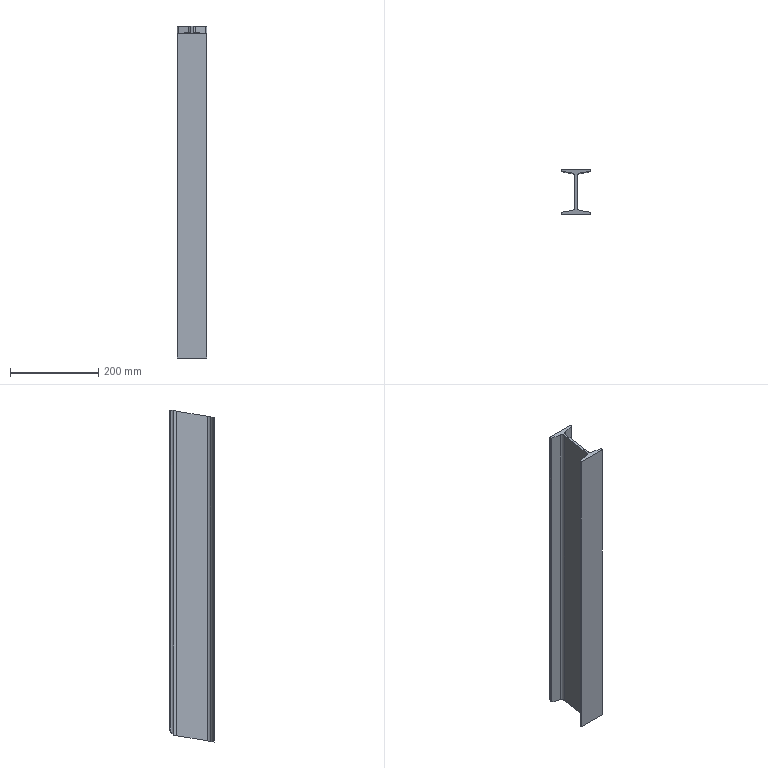Part | SolidWorks | features BaseBody 1 | 1 solid | 23 faces | box 67.6 x 101.6 x 753.5 mm | volume 1021639 mm3 | plane 15 | cylinder 8 | commonest cylinder face diameters 5.6 x4 14.8 x4
STEP:
#1=CARTESIAN_POINT('',(17.268,-1.81,2.654));
#2=VERTEX_POINT('',#1);
#3=CARTESIAN_POINT('',(17.268,68.07,14.348));
#4=VERTEX_POINT('',#3);
#5=CARTESIAN_POINT('',(17.268,-1.81,2.654));
#6=DIRECTION('',(0.,0.9863,0.165));
#7=VECTOR('',#6,1000.);
#8=LINE('',#5,#7);
#9=EDGE_CURVE('',#2,#4,#8,.T.);
#10=ORIENTED_EDGE('',*,*,#9,.T.);
#11=CARTESIAN_POINT('',(17.268,68.07,750.846));
#12=VERTEX_POINT('',#11);
#13=CARTESIAN_POINT('',(17.268,68.07,0.));
#14=DIRECTION('',(0.,0.,1.));
#15=VECTOR('',#14,1000.);
#16=LINE('',#13,#15);
#17=EDGE_CURVE('',#4,#12,#16,.T.);
#18=ORIENTED_EDGE('',*,*,#17,.T.);
#19=CARTESIAN_POINT('',(17.268,-1.81,739.152));
#20=VERTEX_POINT('',#19);
#21=CARTESIAN_POINT('',(17.268,68.07,750.846));
#22=DIRECTION('',(0.,-0.9863,-0.165));
#23=VECTOR('',#22,1000.);
#24=LINE('',#21,#23);
#25=EDGE_CURVE('',#12,#20,#24,.T.);
#26=ORIENTED_EDGE('',*,*,#25,.T.);
#27=CARTESIAN_POINT('',(17.268,-1.81,0.));
#28=DIRECTION('',(0.,0.,-1.));
#29=VECTOR('',#28,1000.);
#30=LINE('',#27,#29);
#31=EDGE_CURVE('',#20,#2,#30,.T.);
#32=ORIENTED_EDGE('',*,*,#31,.T.);
#33=EDGE_LOOP('',(#10,#18,#26,#32));
#34=FACE_OUTER_BOUND('',#33,.T.);
#35=CARTESIAN_POINT('',(17.268,68.07,0.));
#36=DIRECTION('',(1.,0.,0.));
#37=DIRECTION('',(0.,0.,-1.));
#38=AXIS2_PLACEMENT_3D('',#35,#36,#37);
#39=PLANE('',#38);
#40=ADVANCED_FACE('',(#34),#39,.T.);
#41=ORIENTED_EDGE('',*,*,#17,.F.);
#42=CARTESIAN_POINT('',(23.446,75.369,15.569));
#43=VERTEX_POINT('',#42);
#44=CARTESIAN_POINT('',(23.446,75.369,15.569));
#45=CARTESIAN_POINT('',(19.713,74.744,15.465));
#46=CARTESIAN_POINT('',(17.268,71.855,14.981));
#47=CARTESIAN_POINT('',(17.268,68.07,14.348));
#48=(BOUNDED_CURVE()B_SPLINE_CURVE(3,(#44,#45,#46,#47),.UNSPECIFIED.,.F.,.T.)B_SPLINE_CURVE_WITH_KNOTS((4,4),(0.1658,1.571),.UNSPECIFIED.)CURVE()GEOMETRIC_REPRESENTATION_ITEM()RATIONAL_B_SPLINE_CURVE((1.,0.8422,0.8422,1.))REPRESENTATION_ITEM(''));
#49=EDGE_CURVE('',#43,#4,#48,.T.);
#50=ORIENTED_EDGE('',*,*,#49,.F.);
#51=CARTESIAN_POINT('',(23.446,75.369,752.067));
#52=VERTEX_POINT('',#51);
#53=CARTESIAN_POINT('',(23.446,75.369,0.));
#54=DIRECTION('',(0.,0.,-1.));
#55=VECTOR('',#54,1000.);
#56=LINE('',#53,#55);
#57=EDGE_CURVE('',#52,#43,#56,.T.);
#58=ORIENTED_EDGE('',*,*,#57,.F.);
#59=CARTESIAN_POINT('',(17.268,68.07,750.846));
#60=CARTESIAN_POINT('',(17.268,71.855,751.479));
#61=CARTESIAN_POINT('',(19.713,74.744,751.963));
#62=CARTESIAN_POINT('',(23.446,75.369,752.067));
#63=(BOUNDED_CURVE()B_SPLINE_CURVE(3,(#59,#60,#61,#62),.UNSPECIFIED.,.F.,.F.)B_SPLINE_CURVE_WITH_KNOTS((4,4),(4.712,6.117),.UNSPECIFIED.)CURVE()GEOMETRIC_REPRESENTATION_ITEM()RATIONAL_B_SPLINE_CURVE((1.,0.8422,0.8422,1.))REPRESENTATION_ITEM(''));
#64=EDGE_CURVE('',#12,#52,#63,.T.);
#65=ORIENTED_EDGE('',*,*,#64,.F.);
#66=EDGE_LOOP('',(#41,#50,#58,#65));
#67=FACE_OUTER_BOUND('',#66,.T.);
#68=CARTESIAN_POINT('',(24.668,68.07,0.));
#69=DIRECTION('',(0.,0.,1.));
#70=DIRECTION('',(1.,0.,0.));
#71=AXIS2_PLACEMENT_3D('',#68,#69,#70);
#72=CYLINDRICAL_SURFACE('',#71,7.4);
#73=ADVANCED_FACE('',(#67),#72,.F.);
#74=CARTESIAN_POINT('',(12.468,68.07,14.348));
#75=VERTEX_POINT('',#74);
#76=CARTESIAN_POINT('',(6.289,75.369,15.569));
#77=VERTEX_POINT('',#76);
#78=CARTESIAN_POINT('',(12.468,68.07,14.348));
#79=CARTESIAN_POINT('',(12.468,71.855,14.981));
#80=CARTESIAN_POINT('',(10.022,74.744,15.465));
#81=CARTESIAN_POINT('',(6.289,75.369,15.569));
#82=(BOUNDED_CURVE()B_SPLINE_CURVE(3,(#78,#79,#80,#81),.UNSPECIFIED.,.F.,.T.)B_SPLINE_CURVE_WITH_KNOTS((4,4),(4.712,6.117),.UNSPECIFIED.)CURVE()GEOMETRIC_REPRESENTATION_ITEM()RATIONAL_B_SPLINE_CURVE((1.,0.8422,0.8422,1.))REPRESENTATION_ITEM(''));
#83=EDGE_CURVE('',#75,#77,#82,.T.);
#84=ORIENTED_EDGE('',*,*,#83,.T.);
#85=CARTESIAN_POINT('',(2.278,76.04,15.682));
#86=VERTEX_POINT('',#85);
#87=CARTESIAN_POINT('',(6.289,75.369,15.569));
#88=DIRECTION('',(-0.9859,0.165,0.02761));
#89=VECTOR('',#88,1000.);
#90=LINE('',#87,#89);
#91=EDGE_CURVE('',#77,#86,#90,.T.);
#92=ORIENTED_EDGE('',*,*,#91,.T.);
#93=CARTESIAN_POINT('',(27.457,76.04,15.682));
#94=VERTEX_POINT('',#93);
#95=CARTESIAN_POINT('',(-2.032,76.04,15.682));
#96=DIRECTION('',(1.,0.,0.));
#97=VECTOR('',#96,1000.);
#98=LINE('',#95,#97);
#99=EDGE_CURVE('',#86,#94,#98,.T.);
#100=ORIENTED_EDGE('',*,*,#99,.T.);
#101=CARTESIAN_POINT('',(27.457,76.04,15.682));
#102=DIRECTION('',(-0.9859,-0.165,-0.02761));
#103=VECTOR('',#102,1000.);
#104=LINE('',#101,#103);
#105=EDGE_CURVE('',#94,#43,#104,.T.);
#106=ORIENTED_EDGE('',*,*,#105,.T.);
#107=ORIENTED_EDGE('',*,*,#49,.T.);
#108=ORIENTED_EDGE('',*,*,#9,.F.);
#109=CARTESIAN_POINT('',(23.446,-9.108,1.433));
#110=VERTEX_POINT('',#109);
#111=CARTESIAN_POINT('',(17.268,-1.81,2.654));
#112=CARTESIAN_POINT('',(17.268,-5.595,2.021));
#113=CARTESIAN_POINT('',(19.713,-8.484,1.537));
#114=CARTESIAN_POINT('',(23.446,-9.108,1.433));
#115=(BOUNDED_CURVE()B_SPLINE_CURVE(3,(#111,#112,#113,#114),.UNSPECIFIED.,.F.,.F.)B_SPLINE_CURVE_WITH_KNOTS((4,4),(1.571,2.976),.UNSPECIFIED.)CURVE()GEOMETRIC_REPRESENTATION_ITEM()RATIONAL_B_SPLINE_CURVE((1.,0.8422,0.8422,1.))REPRESENTATION_ITEM(''));
#116=EDGE_CURVE('',#2,#110,#115,.T.);
#117=ORIENTED_EDGE('',*,*,#116,.T.);
#118=CARTESIAN_POINT('',(46.33,-12.938,0.7919));
#119=VERTEX_POINT('',#118);
#120=CARTESIAN_POINT('',(23.446,-9.108,1.433));
#121=DIRECTION('',(0.9859,-0.165,-0.02761));
#122=VECTOR('',#121,1000.);
#123=LINE('',#120,#122);
#124=EDGE_CURVE('',#110,#119,#123,.T.);
#125=ORIENTED_EDGE('',*,*,#124,.T.);
#126=CARTESIAN_POINT('',(48.668,-15.699,0.3297));
#127=VERTEX_POINT('',#126);
#128=CARTESIAN_POINT('',(46.33,-12.938,0.7919));
#129=CARTESIAN_POINT('',(47.742,-13.174,0.7523));
#130=CARTESIAN_POINT('',(48.668,-14.267,0.5694));
#131=CARTESIAN_POINT('',(48.668,-15.699,0.3297));
#132=(BOUNDED_CURVE()B_SPLINE_CURVE(3,(#128,#129,#130,#131),.UNSPECIFIED.,.F.,.F.)B_SPLINE_CURVE_WITH_KNOTS((4,4),(0.1658,1.571),.UNSPECIFIED.)CURVE()GEOMETRIC_REPRESENTATION_ITEM()RATIONAL_B_SPLINE_CURVE((1.,0.8422,0.8422,1.))REPRESENTATION_ITEM(''));
#133=EDGE_CURVE('',#119,#127,#132,.T.);
#134=ORIENTED_EDGE('',*,*,#133,.T.);
#135=CARTESIAN_POINT('',(48.668,-17.67,0.));
#136=VERTEX_POINT('',#135);
#137=CARTESIAN_POINT('',(48.668,33.13,8.501));
#138=DIRECTION('',(0.,-0.9863,-0.165));
#139=VECTOR('',#138,1000.);
#140=LINE('',#137,#139);
#141=EDGE_CURVE('',#127,#136,#140,.T.);
#142=ORIENTED_EDGE('',*,*,#141,.T.);
#143=CARTESIAN_POINT('',(-18.932,-17.67,0.));
#144=VERTEX_POINT('',#143);
#145=CARTESIAN_POINT('',(-2.032,-17.67,0.));
#146=DIRECTION('',(-1.,0.,0.));
#147=VECTOR('',#146,1000.);
#148=LINE('',#145,#147);
#149=EDGE_CURVE('',#136,#144,#148,.T.);
#150=ORIENTED_EDGE('',*,*,#149,.T.);
#151=CARTESIAN_POINT('',(-18.932,-15.699,0.3297));
#152=VERTEX_POINT('',#151);
#153=CARTESIAN_POINT('',(-18.932,33.13,8.501));
#154=DIRECTION('',(0.,0.9863,0.165));
#155=VECTOR('',#154,1000.);
#156=LINE('',#153,#155);
#157=EDGE_CURVE('',#144,#152,#156,.T.);
#158=ORIENTED_EDGE('',*,*,#157,.T.);
#159=CARTESIAN_POINT('',(-16.594,-12.938,0.7919));
#160=VERTEX_POINT('',#159);
#161=CARTESIAN_POINT('',(-18.932,-15.699,0.3297));
#162=CARTESIAN_POINT('',(-18.932,-14.267,0.5694));
#163=CARTESIAN_POINT('',(-18.007,-13.174,0.7523));
#164=CARTESIAN_POINT('',(-16.594,-12.938,0.7919));
#165=(BOUNDED_CURVE()B_SPLINE_CURVE(3,(#161,#162,#163,#164),.UNSPECIFIED.,.F.,.F.)B_SPLINE_CURVE_WITH_KNOTS((4,4),(4.712,6.117),.UNSPECIFIED.)CURVE()GEOMETRIC_REPRESENTATION_ITEM()RATIONAL_B_SPLINE_CURVE((1.,0.8422,0.8422,1.))REPRESENTATION_ITEM(''));
#166=EDGE_CURVE('',#152,#160,#165,.T.);
#167=ORIENTED_EDGE('',*,*,#166,.T.);
#168=CARTESIAN_POINT('',(6.289,-9.108,1.433));
#169=VERTEX_POINT('',#168);
#170=CARTESIAN_POINT('',(-16.594,-12.938,0.7919));
#171=DIRECTION('',(0.9859,0.165,0.02761));
#172=VECTOR('',#171,1000.);
#173=LINE('',#170,#172);
#174=EDGE_CURVE('',#160,#169,#173,.T.);
#175=ORIENTED_EDGE('',*,*,#174,.T.);
#176=CARTESIAN_POINT('',(12.468,-1.81,2.654));
#177=VERTEX_POINT('',#176);
#178=CARTESIAN_POINT('',(6.289,-9.108,1.433));
#179=CARTESIAN_POINT('',(10.022,-8.484,1.537));
#180=CARTESIAN_POINT('',(12.468,-5.595,2.021));
#181=CARTESIAN_POINT('',(12.468,-1.81,2.654));
#182=(BOUNDED_CURVE()B_SPLINE_CURVE(3,(#178,#179,#180,#181),.UNSPECIFIED.,.F.,.T.)B_SPLINE_CURVE_WITH_KNOTS((4,4),(3.307,4.712),.UNSPECIFIED.)CURVE()GEOMETRIC_REPRESENTATION_ITEM()RATIONAL_B_SPLINE_CURVE((1.,0.8422,0.8422,1.))REPRESENTATION_ITEM(''));
#183=EDGE_CURVE('',#169,#177,#182,.T.);
#184=ORIENTED_EDGE('',*,*,#183,.T.);
#185=CARTESIAN_POINT('',(12.468,33.13,8.501));
#186=DIRECTION('',(0.,0.9863,0.165));
#187=VECTOR('',#186,1000.);
#188=LINE('',#185,#187);
#189=EDGE_CURVE('',#177,#75,#188,.T.);
#190=ORIENTED_EDGE('',*,*,#189,.T.);
#191=EDGE_LOOP('',(#84,#92,#100,#106,#107,#108,#117,#125,#134,#142,#150,#158,#167,#175,#184,#190));
#192=FACE_OUTER_BOUND('',#191,.T.);
#193=CARTESIAN_POINT('',(-2.032,33.13,8.501));
#194=DIRECTION('',(0.,0.165,-0.9863));
#195=DIRECTION('',(0.,0.9863,0.165));
#196=AXIS2_PLACEMENT_3D('',#193,#194,#195);
#197=PLANE('',#196);
#198=ADVANCED_FACE('',(#192),#197,.T.);
#199=CARTESIAN_POINT('',(23.446,-9.108,737.931));
#200=VERTEX_POINT('',#199);
#201=CARTESIAN_POINT('',(23.446,-9.108,0.));
#202=DIRECTION('',(0.,0.,1.));
#203=VECTOR('',#202,1000.);
#204=LINE('',#201,#203);
#205=EDGE_CURVE('',#110,#200,#204,.T.);
#206=ORIENTED_EDGE('',*,*,#205,.F.);
#207=ORIENTED_EDGE('',*,*,#116,.F.);
#208=ORIENTED_EDGE('',*,*,#31,.F.);
#209=CARTESIAN_POINT('',(23.446,-9.108,737.931));
#210=CARTESIAN_POINT('',(19.713,-8.484,738.035));
#211=CARTESIAN_POINT('',(17.268,-5.595,738.519));
#212=CARTESIAN_POINT('',(17.268,-1.81,739.152));
#213=(BOUNDED_CURVE()B_SPLINE_CURVE(3,(#209,#210,#211,#212),.UNSPECIFIED.,.F.,.T.)B_SPLINE_CURVE_WITH_KNOTS((4,4),(3.307,4.712),.UNSPECIFIED.)CURVE()GEOMETRIC_REPRESENTATION_ITEM()RATIONAL_B_SPLINE_CURVE((1.,0.8422,0.8422,1.))REPRESENTATION_ITEM(''));
#214=EDGE_CURVE('',#200,#20,#213,.T.);
#215=ORIENTED_EDGE('',*,*,#214,.F.);
#216=EDGE_LOOP('',(#206,#207,#208,#215));
#217=FACE_OUTER_BOUND('',#216,.T.);
#218=CARTESIAN_POINT('',(24.668,-1.81,0.));
#219=DIRECTION('',(0.,0.,1.));
#220=DIRECTION('',(1.,0.,0.));
#221=AXIS2_PLACEMENT_3D('',#218,#219,#220);
#222=CYLINDRICAL_SURFACE('',#221,7.4);
#223=ADVANCED_FACE('',(#217),#222,.F.);
#224=CARTESIAN_POINT('',(6.289,-9.108,737.931));
#225=VERTEX_POINT('',#224);
#226=CARTESIAN_POINT('',(-16.594,-12.938,737.29));
#227=VERTEX_POINT('',#226);
#228=CARTESIAN_POINT('',(6.289,-9.108,737.931));
#229=DIRECTION('',(-0.9859,-0.165,-0.02761));
#230=VECTOR('',#229,1000.);
#231=LINE('',#228,#230);
#232=EDGE_CURVE('',#225,#227,#231,.T.);
#233=ORIENTED_EDGE('',*,*,#232,.T.);
#234=CARTESIAN_POINT('',(-18.932,-15.699,736.828));
#235=VERTEX_POINT('',#234);
#236=CARTESIAN_POINT('',(-16.594,-12.938,737.29));
#237=CARTESIAN_POINT('',(-18.007,-13.174,737.25));
#238=CARTESIAN_POINT('',(-18.932,-14.267,737.067));
#239=CARTESIAN_POINT('',(-18.932,-15.699,736.828));
#240=(BOUNDED_CURVE()B_SPLINE_CURVE(3,(#236,#237,#238,#239),.UNSPECIFIED.,.F.,.T.)B_SPLINE_CURVE_WITH_KNOTS((4,4),(0.1658,1.571),.UNSPECIFIED.)CURVE()GEOMETRIC_REPRESENTATION_ITEM()RATIONAL_B_SPLINE_CURVE((1.,0.8422,0.8422,1.))REPRESENTATION_ITEM(''));
#241=EDGE_CURVE('',#227,#235,#240,.T.);
#242=ORIENTED_EDGE('',*,*,#241,.T.);
#243=CARTESIAN_POINT('',(-18.932,-17.67,736.498));
#244=VERTEX_POINT('',#243);
#245=CARTESIAN_POINT('',(-18.932,33.13,744.999));
#246=DIRECTION('',(0.,-0.9863,-0.165));
#247=VECTOR('',#246,1000.);
#248=LINE('',#245,#247);
#249=EDGE_CURVE('',#235,#244,#248,.T.);
#250=ORIENTED_EDGE('',*,*,#249,.T.);
#251=CARTESIAN_POINT('',(48.668,-17.67,736.498));
#252=VERTEX_POINT('',#251);
#253=CARTESIAN_POINT('',(31.768,-17.67,736.498));
#254=DIRECTION('',(1.,0.,0.));
#255=VECTOR('',#254,1000.);
#256=LINE('',#253,#255);
#257=EDGE_CURVE('',#244,#252,#256,.T.);
#258=ORIENTED_EDGE('',*,*,#257,.T.);
#259=CARTESIAN_POINT('',(48.668,-15.699,736.828));
#260=VERTEX_POINT('',#259);
#261=CARTESIAN_POINT('',(48.668,33.13,744.999));
#262=DIRECTION('',(0.,0.9863,0.165));
#263=VECTOR('',#262,1000.);
#264=LINE('',#261,#263);
#265=EDGE_CURVE('',#252,#260,#264,.T.);
#266=ORIENTED_EDGE('',*,*,#265,.T.);
#267=CARTESIAN_POINT('',(46.33,-12.938,737.29));
#268=VERTEX_POINT('',#267);
#269=CARTESIAN_POINT('',(48.668,-15.699,736.828));
#270=CARTESIAN_POINT('',(48.668,-14.267,737.067));
#271=CARTESIAN_POINT('',(47.742,-13.174,737.25));
#272=CARTESIAN_POINT('',(46.33,-12.938,737.29));
#273=(BOUNDED_CURVE()B_SPLINE_CURVE(3,(#269,#270,#271,#272),.UNSPECIFIED.,.F.,.T.)B_SPLINE_CURVE_WITH_KNOTS((4,4),(4.712,6.117),.UNSPECIFIED.)CURVE()GEOMETRIC_REPRESENTATION_ITEM()RATIONAL_B_SPLINE_CURVE((1.,0.8422,0.8422,1.))REPRESENTATION_ITEM(''));
#274=EDGE_CURVE('',#260,#268,#273,.T.);
#275=ORIENTED_EDGE('',*,*,#274,.T.);
#276=CARTESIAN_POINT('',(46.33,-12.938,737.29));
#277=DIRECTION('',(-0.9859,0.165,0.02761));
#278=VECTOR('',#277,1000.);
#279=LINE('',#276,#278);
#280=EDGE_CURVE('',#268,#200,#279,.T.);
#281=ORIENTED_EDGE('',*,*,#280,.T.);
#282=ORIENTED_EDGE('',*,*,#214,.T.);
#283=ORIENTED_EDGE('',*,*,#25,.F.);
#284=ORIENTED_EDGE('',*,*,#64,.T.);
#285=CARTESIAN_POINT('',(46.33,79.198,752.708));
#286=VERTEX_POINT('',#285);
#287=CARTESIAN_POINT('',(23.446,75.369,752.067));
#288=DIRECTION('',(0.9859,0.165,0.02761));
#289=VECTOR('',#288,1000.);
#290=LINE('',#287,#289);
#291=EDGE_CURVE('',#52,#286,#290,.T.);
#292=ORIENTED_EDGE('',*,*,#291,.T.);
#293=CARTESIAN_POINT('',(48.668,81.96,753.17));
#294=VERTEX_POINT('',#293);
#295=CARTESIAN_POINT('',(46.33,79.198,752.708));
#296=CARTESIAN_POINT('',(47.742,79.434,752.748));
#297=CARTESIAN_POINT('',(48.668,80.527,752.931));
#298=CARTESIAN_POINT('',(48.668,81.96,753.17));
#299=(BOUNDED_CURVE()B_SPLINE_CURVE(3,(#295,#296,#297,#298),.UNSPECIFIED.,.F.,.T.)B_SPLINE_CURVE_WITH_KNOTS((4,4),(3.307,4.712),.UNSPECIFIED.)CURVE()GEOMETRIC_REPRESENTATION_ITEM()RATIONAL_B_SPLINE_CURVE((1.,0.8422,0.8422,1.))REPRESENTATION_ITEM(''));
#300=EDGE_CURVE('',#286,#294,#299,.T.);
#301=ORIENTED_EDGE('',*,*,#300,.T.);
#302=CARTESIAN_POINT('',(48.668,83.93,753.5));
#303=VERTEX_POINT('',#302);
#304=CARTESIAN_POINT('',(48.668,33.13,744.999));
#305=DIRECTION('',(0.,0.9863,0.165));
#306=VECTOR('',#305,1000.);
#307=LINE('',#304,#306);
#308=EDGE_CURVE('',#294,#303,#307,.T.);
#309=ORIENTED_EDGE('',*,*,#308,.T.);
#310=CARTESIAN_POINT('',(-18.932,83.93,753.5));
#311=VERTEX_POINT('',#310);
#312=CARTESIAN_POINT('',(31.768,83.93,753.5));
#313=DIRECTION('',(-1.,0.,0.));
#314=VECTOR('',#313,1000.);
#315=LINE('',#312,#314);
#316=EDGE_CURVE('',#303,#311,#315,.T.);
#317=ORIENTED_EDGE('',*,*,#316,.T.);
#318=CARTESIAN_POINT('',(-18.932,81.96,753.17));
#319=VERTEX_POINT('',#318);
#320=CARTESIAN_POINT('',(-18.932,33.13,744.999));
#321=DIRECTION('',(0.,-0.9863,-0.165));
#322=VECTOR('',#321,1000.);
#323=LINE('',#320,#322);
#324=EDGE_CURVE('',#311,#319,#323,.T.);
#325=ORIENTED_EDGE('',*,*,#324,.T.);
#326=CARTESIAN_POINT('',(-16.594,79.198,752.708));
#327=VERTEX_POINT('',#326);
#328=CARTESIAN_POINT('',(-18.932,81.96,753.17));
#329=CARTESIAN_POINT('',(-18.932,80.527,752.931));
#330=CARTESIAN_POINT('',(-18.007,79.434,752.748));
#331=CARTESIAN_POINT('',(-16.594,79.198,752.708));
#332=(BOUNDED_CURVE()B_SPLINE_CURVE(3,(#328,#329,#330,#331),.UNSPECIFIED.,.F.,.T.)B_SPLINE_CURVE_WITH_KNOTS((4,4),(1.571,2.976),.UNSPECIFIED.)CURVE()GEOMETRIC_REPRESENTATION_ITEM()RATIONAL_B_SPLINE_CURVE((1.,0.8422,0.8422,1.))REPRESENTATION_ITEM(''));
#333=EDGE_CURVE('',#319,#327,#332,.T.);
#334=ORIENTED_EDGE('',*,*,#333,.T.);
#335=CARTESIAN_POINT('',(6.289,75.369,752.067));
#336=VERTEX_POINT('',#335);
#337=CARTESIAN_POINT('',(-16.594,79.198,752.708));
#338=DIRECTION('',(0.9859,-0.165,-0.02761));
#339=VECTOR('',#338,1000.);
#340=LINE('',#337,#339);
#341=EDGE_CURVE('',#327,#336,#340,.T.);
#342=ORIENTED_EDGE('',*,*,#341,.T.);
#343=CARTESIAN_POINT('',(12.468,68.07,750.846));
#344=VERTEX_POINT('',#343);
#345=CARTESIAN_POINT('',(6.289,75.369,752.067));
#346=CARTESIAN_POINT('',(10.022,74.744,751.963));
#347=CARTESIAN_POINT('',(12.468,71.855,751.479));
#348=CARTESIAN_POINT('',(12.468,68.07,750.846));
#349=(BOUNDED_CURVE()B_SPLINE_CURVE(3,(#345,#346,#347,#348),.UNSPECIFIED.,.F.,.T.)B_SPLINE_CURVE_WITH_KNOTS((4,4),(0.1658,1.571),.UNSPECIFIED.)CURVE()GEOMETRIC_REPRESENTATION_ITEM()RATIONAL_B_SPLINE_CURVE((1.,0.8422,0.8422,1.))REPRESENTATION_ITEM(''));
#350=EDGE_CURVE('',#336,#344,#349,.T.);
#351=ORIENTED_EDGE('',*,*,#350,.T.);
#352=CARTESIAN_POINT('',(12.468,-1.81,739.152));
#353=VERTEX_POINT('',#352);
#354=CARTESIAN_POINT('',(12.468,33.13,744.999));
#355=DIRECTION('',(0.,-0.9863,-0.165));
#356=VECTOR('',#355,1000.);
#357=LINE('',#354,#356);
#358=EDGE_CURVE('',#344,#353,#357,.T.);
#359=ORIENTED_EDGE('',*,*,#358,.T.);
#360=CARTESIAN_POINT('',(12.468,-1.81,739.152));
#361=CARTESIAN_POINT('',(12.468,-5.595,738.519));
#362=CARTESIAN_POINT('',(10.022,-8.484,738.035));
#363=CARTESIAN_POINT('',(6.289,-9.108,737.931));
#364=(BOUNDED_CURVE()B_SPLINE_CURVE(3,(#360,#361,#362,#363),.UNSPECIFIED.,.F.,.T.)B_SPLINE_CURVE_WITH_KNOTS((4,4),(1.571,2.976),.UNSPECIFIED.)CURVE()GEOMETRIC_REPRESENTATION_ITEM()RATIONAL_B_SPLINE_CURVE((1.,0.8422,0.8422,1.))REPRESENTATION_ITEM(''));
#365=EDGE_CURVE('',#353,#225,#364,.T.);
#366=ORIENTED_EDGE('',*,*,#365,.T.);
#367=EDGE_LOOP('',(#233,#242,#250,#258,#266,#275,#281,#282,#283,#284,#292,#301,#309,#317,#325,#334,#342,#351,#359,#366));
#368=FACE_OUTER_BOUND('',#367,.T.);
#369=CARTESIAN_POINT('',(31.768,33.13,744.999));
#370=DIRECTION('',(0.,-0.165,0.9863));
#371=DIRECTION('',(0.,-0.9863,-0.165));
#372=AXIS2_PLACEMENT_3D('',#369,#370,#371);
#373=PLANE('',#372);
#374=ADVANCED_FACE('',(#368),#373,.T.);
#375=ORIENTED_EDGE('',*,*,#57,.T.);
#376=ORIENTED_EDGE('',*,*,#105,.F.);
#377=CARTESIAN_POINT('',(46.33,79.198,19.412));
#378=VERTEX_POINT('',#377);
#379=CARTESIAN_POINT('',(27.457,76.04,15.682));
#380=DIRECTION('',(0.9681,0.162,0.1914));
#381=VECTOR('',#380,1000.);
#382=LINE('',#379,#381);
#383=EDGE_CURVE('',#94,#378,#382,.T.);
#384=ORIENTED_EDGE('',*,*,#383,.T.);
#385=CARTESIAN_POINT('',(46.33,79.198,0.));
#386=DIRECTION('',(0.,0.,1.));
#387=VECTOR('',#386,1000.);
#388=LINE('',#385,#387);
#389=EDGE_CURVE('',#378,#286,#388,.T.);
#390=ORIENTED_EDGE('',*,*,#389,.T.);
#391=ORIENTED_EDGE('',*,*,#291,.F.);
#392=EDGE_LOOP('',(#375,#376,#384,#390,#391));
#393=FACE_OUTER_BOUND('',#392,.T.);
#394=CARTESIAN_POINT('',(46.33,79.198,0.));
#395=DIRECTION('',(0.165,-0.9863,0.));
#396=DIRECTION('',(0.9863,0.165,0.));
#397=AXIS2_PLACEMENT_3D('',#394,#395,#396);
#398=PLANE('',#397);
#399=ADVANCED_FACE('',(#393),#398,.T.);
#400=ORIENTED_EDGE('',*,*,#341,.F.);
#401=CARTESIAN_POINT('',(-16.594,79.198,19.412));
#402=VERTEX_POINT('',#401);
#403=CARTESIAN_POINT('',(-16.594,79.198,0.));
#404=DIRECTION('',(0.,0.,-1.));
#405=VECTOR('',#404,1000.);
#406=LINE('',#403,#405);
#407=EDGE_CURVE('',#327,#402,#406,.T.);
#408=ORIENTED_EDGE('',*,*,#407,.T.);
#409=CARTESIAN_POINT('',(-16.594,79.198,19.412));
#410=DIRECTION('',(0.9681,-0.162,-0.1914));
#411=VECTOR('',#410,1000.);
#412=LINE('',#409,#411);
#413=EDGE_CURVE('',#402,#86,#412,.T.);
#414=ORIENTED_EDGE('',*,*,#413,.T.);
#415=ORIENTED_EDGE('',*,*,#91,.F.);
#416=CARTESIAN_POINT('',(6.289,75.369,0.));
#417=DIRECTION('',(0.,0.,1.));
#418=VECTOR('',#417,1000.);
#419=LINE('',#416,#418);
#420=EDGE_CURVE('',#77,#336,#419,.T.);
#421=ORIENTED_EDGE('',*,*,#420,.T.);
#422=EDGE_LOOP('',(#400,#408,#414,#415,#421));
#423=FACE_OUTER_BOUND('',#422,.T.);
#424=CARTESIAN_POINT('',(6.289,75.369,0.));
#425=DIRECTION('',(-0.165,-0.9863,0.));
#426=DIRECTION('',(0.9863,-0.165,0.));
#427=AXIS2_PLACEMENT_3D('',#424,#425,#426);
#428=PLANE('',#427);
#429=ADVANCED_FACE('',(#423),#428,.T.);
#430=ORIENTED_EDGE('',*,*,#420,.F.);
#431=ORIENTED_EDGE('',*,*,#83,.F.);
#432=CARTESIAN_POINT('',(12.468,68.07,0.));
#433=DIRECTION('',(0.,0.,-1.));
#434=VECTOR('',#433,1000.);
#435=LINE('',#432,#434);
#436=EDGE_CURVE('',#344,#75,#435,.T.);
#437=ORIENTED_EDGE('',*,*,#436,.F.);
#438=ORIENTED_EDGE('',*,*,#350,.F.);
#439=EDGE_LOOP('',(#430,#431,#437,#438));
#440=FACE_OUTER_BOUND('',#439,.T.);
#441=CARTESIAN_POINT('',(5.068,68.07,0.));
#442=DIRECTION('',(0.,0.,1.));
#443=DIRECTION('',(1.,0.,0.));
#444=AXIS2_PLACEMENT_3D('',#441,#442,#443);
#445=CYLINDRICAL_SURFACE('',#444,7.4);
#446=ADVANCED_FACE('',(#440),#445,.F.);
#447=ORIENTED_EDGE('',*,*,#189,.F.);
#448=CARTESIAN_POINT('',(12.468,-1.81,0.));
#449=DIRECTION('',(0.,0.,1.));
#450=VECTOR('',#449,1000.);
#451=LINE('',#448,#450);
#452=EDGE_CURVE('',#177,#353,#451,.T.);
#453=ORIENTED_EDGE('',*,*,#452,.T.);
#454=ORIENTED_EDGE('',*,*,#358,.F.);
#455=ORIENTED_EDGE('',*,*,#436,.T.);
#456=EDGE_LOOP('',(#447,#453,#454,#455));
#457=FACE_OUTER_BOUND('',#456,.T.);
#458=CARTESIAN_POINT('',(12.468,-1.81,0.));
#459=DIRECTION('',(-1.,0.,0.));
#460=DIRECTION('',(0.,0.,1.));
#461=AXIS2_PLACEMENT_3D('',#458,#459,#460);
#462=PLANE('',#461);
#463=ADVANCED_FACE('',(#457),#462,.T.);
#464=ORIENTED_EDGE('',*,*,#452,.F.);
#465=ORIENTED_EDGE('',*,*,#183,.F.);
#466=CARTESIAN_POINT('',(6.289,-9.108,0.));
#467=DIRECTION('',(0.,0.,-1.));
#468=VECTOR('',#467,1000.);
#469=LINE('',#466,#468);
#470=EDGE_CURVE('',#225,#169,#469,.T.);
#471=ORIENTED_EDGE('',*,*,#470,.F.);
#472=ORIENTED_EDGE('',*,*,#365,.F.);
#473=EDGE_LOOP('',(#464,#465,#471,#472));
#474=FACE_OUTER_BOUND('',#473,.T.);
#475=CARTESIAN_POINT('',(5.068,-1.81,0.));
#476=DIRECTION('',(0.,0.,1.));
#477=DIRECTION('',(1.,0.,0.));
#478=AXIS2_PLACEMENT_3D('',#475,#476,#477);
#479=CYLINDRICAL_SURFACE('',#478,7.4);
#480=ADVANCED_FACE('',(#474),#479,.F.);
#481=ORIENTED_EDGE('',*,*,#174,.F.);
#482=CARTESIAN_POINT('',(-16.594,-12.938,0.));
#483=DIRECTION('',(0.,0.,1.));
#484=VECTOR('',#483,1000.);
#485=LINE('',#482,#484);
#486=EDGE_CURVE('',#160,#227,#485,.T.);
#487=ORIENTED_EDGE('',*,*,#486,.T.);
#488=ORIENTED_EDGE('',*,*,#232,.F.);
#489=ORIENTED_EDGE('',*,*,#470,.T.);
#490=EDGE_LOOP('',(#481,#487,#488,#489));
#491=FACE_OUTER_BOUND('',#490,.T.);
#492=CARTESIAN_POINT('',(-16.594,-12.938,0.));
#493=DIRECTION('',(-0.165,0.9863,0.));
#494=DIRECTION('',(-0.9863,-0.165,0.));
#495=AXIS2_PLACEMENT_3D('',#492,#493,#494);
#496=PLANE('',#495);
#497=ADVANCED_FACE('',(#491),#496,.T.);
#498=ORIENTED_EDGE('',*,*,#166,.F.);
#499=CARTESIAN_POINT('',(-18.932,-15.699,0.));
#500=DIRECTION('',(0.,0.,1.));
#501=VECTOR('',#500,1000.);
#502=LINE('',#499,#501);
#503=EDGE_CURVE('',#152,#235,#502,.T.);
#504=ORIENTED_EDGE('',*,*,#503,.T.);
#505=ORIENTED_EDGE('',*,*,#241,.F.);
#506=ORIENTED_EDGE('',*,*,#486,.F.);
#507=EDGE_LOOP('',(#498,#504,#505,#506));
#508=FACE_OUTER_BOUND('',#507,.T.);
#509=CARTESIAN_POINT('',(-16.132,-15.699,0.));
#510=DIRECTION('',(0.,0.,1.));
#511=DIRECTION('',(1.,0.,0.));
#512=AXIS2_PLACEMENT_3D('',#509,#510,#511);
#513=CYLINDRICAL_SURFACE('',#512,2.8);
#514=ADVANCED_FACE('',(#508),#513,.T.);
#515=ORIENTED_EDGE('',*,*,#157,.F.);
#516=CARTESIAN_POINT('',(-18.932,-17.67,0.));
#517=DIRECTION('',(0.,0.,1.));
#518=VECTOR('',#517,1000.);
#519=LINE('',#516,#518);
#520=EDGE_CURVE('',#144,#244,#519,.T.);
#521=ORIENTED_EDGE('',*,*,#520,.T.);
#522=ORIENTED_EDGE('',*,*,#249,.F.);
#523=ORIENTED_EDGE('',*,*,#503,.F.);
#524=EDGE_LOOP('',(#515,#521,#522,#523));
#525=FACE_OUTER_BOUND('',#524,.T.);
#526=CARTESIAN_POINT('',(-18.932,-17.67,0.));
#527=DIRECTION('',(-1.,0.,0.));
#528=DIRECTION('',(0.,0.,1.));
#529=AXIS2_PLACEMENT_3D('',#526,#527,#528);
#530=PLANE('',#529);
#531=ADVANCED_FACE('',(#525),#530,.T.);
#532=ORIENTED_EDGE('',*,*,#149,.F.);
#533=CARTESIAN_POINT('',(48.668,-17.67,0.));
#534=DIRECTION('',(0.,0.,1.));
#535=VECTOR('',#534,1000.);
#536=LINE('',#533,#535);
#537=EDGE_CURVE('',#136,#252,#536,.T.);
#538=ORIENTED_EDGE('',*,*,#537,.T.);
#539=ORIENTED_EDGE('',*,*,#257,.F.);
#540=ORIENTED_EDGE('',*,*,#520,.F.);
#541=EDGE_LOOP('',(#532,#538,#539,#540));
#542=FACE_OUTER_BOUND('',#541,.T.);
#543=CARTESIAN_POINT('',(48.668,-17.67,0.));
#544=DIRECTION('',(0.,-1.,0.));
#545=DIRECTION('',(0.,0.,-1.));
#546=AXIS2_PLACEMENT_3D('',#543,#544,#545);
#547=PLANE('',#546);
#548=ADVANCED_FACE('',(#542),#547,.T.);
#549=ORIENTED_EDGE('',*,*,#141,.F.);
#550=CARTESIAN_POINT('',(48.668,-15.699,0.));
#551=DIRECTION('',(0.,0.,1.));
#552=VECTOR('',#551,1000.);
#553=LINE('',#550,#552);
#554=EDGE_CURVE('',#127,#260,#553,.T.);
#555=ORIENTED_EDGE('',*,*,#554,.T.);
#556=ORIENTED_EDGE('',*,*,#265,.F.);
#557=ORIENTED_EDGE('',*,*,#537,.F.);
#558=EDGE_LOOP('',(#549,#555,#556,#557));
#559=FACE_OUTER_BOUND('',#558,.T.);
#560=CARTESIAN_POINT('',(48.668,-15.699,0.));
#561=DIRECTION('',(1.,0.,0.));
#562=DIRECTION('',(0.,0.,-1.));
#563=AXIS2_PLACEMENT_3D('',#560,#561,#562);
#564=PLANE('',#563);
#565=ADVANCED_FACE('',(#559),#564,.T.);
#566=ORIENTED_EDGE('',*,*,#133,.F.);
#567=CARTESIAN_POINT('',(46.33,-12.938,0.));
#568=DIRECTION('',(0.,0.,1.));
#569=VECTOR('',#568,1000.);
#570=LINE('',#567,#569);
#571=EDGE_CURVE('',#119,#268,#570,.T.);
#572=ORIENTED_EDGE('',*,*,#571,.T.);
#573=ORIENTED_EDGE('',*,*,#274,.F.);
#574=ORIENTED_EDGE('',*,*,#554,.F.);
#575=EDGE_LOOP('',(#566,#572,#573,#574));
#576=FACE_OUTER_BOUND('',#575,.T.);
#577=CARTESIAN_POINT('',(45.868,-15.699,0.));
#578=DIRECTION('',(0.,0.,1.));
#579=DIRECTION('',(1.,0.,0.));
#580=AXIS2_PLACEMENT_3D('',#577,#578,#579);
#581=CYLINDRICAL_SURFACE('',#580,2.8);
#582=ADVANCED_FACE('',(#576),#581,.T.);
#583=ORIENTED_EDGE('',*,*,#124,.F.);
#584=ORIENTED_EDGE('',*,*,#205,.T.);
#585=ORIENTED_EDGE('',*,*,#280,.F.);
#586=ORIENTED_EDGE('',*,*,#571,.F.);
#587=EDGE_LOOP('',(#583,#584,#585,#586));
#588=FACE_OUTER_BOUND('',#587,.T.);
#589=CARTESIAN_POINT('',(23.446,-9.108,0.));
#590=DIRECTION('',(0.165,0.9863,0.));
#591=DIRECTION('',(-0.9863,0.165,0.));
#592=AXIS2_PLACEMENT_3D('',#589,#590,#591);
#593=PLANE('',#592);
#594=ADVANCED_FACE('',(#588),#593,.T.);
#595=CARTESIAN_POINT('',(48.668,83.93,25.002));
#596=VERTEX_POINT('',#595);
#597=CARTESIAN_POINT('',(48.668,81.96,22.674));
#598=VERTEX_POINT('',#597);
#599=CARTESIAN_POINT('',(48.668,79.985,20.342));
#600=DIRECTION('',(0.,-0.6461,-0.7632));
#601=VECTOR('',#600,1000.);
#602=LINE('',#599,#601);
#603=EDGE_CURVE('',#596,#598,#602,.T.);
#604=ORIENTED_EDGE('',*,*,#603,.T.);
#605=CARTESIAN_POINT('',(48.668,81.96,22.674));
#606=CARTESIAN_POINT('',(48.668,80.527,20.983));
#607=CARTESIAN_POINT('',(47.742,79.434,19.691));
#608=CARTESIAN_POINT('',(46.33,79.198,19.412));
#609=(BOUNDED_CURVE()B_SPLINE_CURVE(3,(#605,#606,#607,#608),.UNSPECIFIED.,.F.,.T.)B_SPLINE_CURVE_WITH_KNOTS((4,4),(1.571,2.976),.UNSPECIFIED.)CURVE()GEOMETRIC_REPRESENTATION_ITEM()RATIONAL_B_SPLINE_CURVE((1.,0.8422,0.8422,1.))REPRESENTATION_ITEM(''));
#610=EDGE_CURVE('',#598,#378,#609,.T.);
#611=ORIENTED_EDGE('',*,*,#610,.T.);
#612=ORIENTED_EDGE('',*,*,#383,.F.);
#613=ORIENTED_EDGE('',*,*,#99,.F.);
#614=ORIENTED_EDGE('',*,*,#413,.F.);
#615=CARTESIAN_POINT('',(-18.932,81.96,22.674));
#616=VERTEX_POINT('',#615);
#617=CARTESIAN_POINT('',(-16.594,79.198,19.412));
#618=CARTESIAN_POINT('',(-18.007,79.434,19.691));
#619=CARTESIAN_POINT('',(-18.932,80.527,20.983));
#620=CARTESIAN_POINT('',(-18.932,81.96,22.674));
#621=(BOUNDED_CURVE()B_SPLINE_CURVE(3,(#617,#618,#619,#620),.UNSPECIFIED.,.F.,.T.)B_SPLINE_CURVE_WITH_KNOTS((4,4),(3.307,4.712),.UNSPECIFIED.)CURVE()GEOMETRIC_REPRESENTATION_ITEM()RATIONAL_B_SPLINE_CURVE((1.,0.8422,0.8422,1.))REPRESENTATION_ITEM(''));
#622=EDGE_CURVE('',#402,#616,#621,.T.);
#623=ORIENTED_EDGE('',*,*,#622,.T.);
#624=CARTESIAN_POINT('',(-18.932,83.93,25.002));
#625=VERTEX_POINT('',#624);
#626=CARTESIAN_POINT('',(-18.932,79.985,20.342));
#627=DIRECTION('',(0.,0.6461,0.7632));
#628=VECTOR('',#627,1000.);
#629=LINE('',#626,#628);
#630=EDGE_CURVE('',#616,#625,#629,.T.);
#631=ORIENTED_EDGE('',*,*,#630,.T.);
#632=CARTESIAN_POINT('',(-10.482,83.93,25.002));
#633=DIRECTION('',(1.,0.,0.));
#634=VECTOR('',#633,1000.);
#635=LINE('',#632,#634);
#636=EDGE_CURVE('',#625,#596,#635,.T.);
#637=ORIENTED_EDGE('',*,*,#636,.T.);
#638=EDGE_LOOP('',(#604,#611,#612,#613,#614,#623,#631,#637));
#639=FACE_OUTER_BOUND('',#638,.T.);
#640=CARTESIAN_POINT('',(-10.482,79.985,20.342));
#641=DIRECTION('',(0.,0.7632,-0.6461));
#642=DIRECTION('',(0.,0.6461,0.7632));
#643=AXIS2_PLACEMENT_3D('',#640,#641,#642);
#644=PLANE('',#643);
#645=ADVANCED_FACE('',(#639),#644,.T.);
#646=ORIENTED_EDGE('',*,*,#333,.F.);
#647=CARTESIAN_POINT('',(-18.932,81.96,0.));
#648=DIRECTION('',(0.,0.,-1.));
#649=VECTOR('',#648,1000.);
#650=LINE('',#647,#649);
#651=EDGE_CURVE('',#319,#616,#650,.T.);
#652=ORIENTED_EDGE('',*,*,#651,.T.);
#653=ORIENTED_EDGE('',*,*,#622,.F.);
#654=ORIENTED_EDGE('',*,*,#407,.F.);
#655=EDGE_LOOP('',(#646,#652,#653,#654));
#656=FACE_OUTER_BOUND('',#655,.T.);
#657=CARTESIAN_POINT('',(-16.132,81.96,0.));
#658=DIRECTION('',(0.,0.,1.));
#659=DIRECTION('',(1.,0.,0.));
#660=AXIS2_PLACEMENT_3D('',#657,#658,#659);
#661=CYLINDRICAL_SURFACE('',#660,2.8);
#662=ADVANCED_FACE('',(#656),#661,.T.);
#663=ORIENTED_EDGE('',*,*,#324,.F.);
#664=CARTESIAN_POINT('',(-18.932,83.93,0.));
#665=DIRECTION('',(0.,0.,-1.));
#666=VECTOR('',#665,1000.);
#667=LINE('',#664,#666);
#668=EDGE_CURVE('',#311,#625,#667,.T.);
#669=ORIENTED_EDGE('',*,*,#668,.T.);
#670=ORIENTED_EDGE('',*,*,#630,.F.);
#671=ORIENTED_EDGE('',*,*,#651,.F.);
#672=EDGE_LOOP('',(#663,#669,#670,#671));
#673=FACE_OUTER_BOUND('',#672,.T.);
#674=CARTESIAN_POINT('',(-18.932,81.96,0.));
#675=DIRECTION('',(-1.,0.,0.));
#676=DIRECTION('',(0.,0.,1.));
#677=AXIS2_PLACEMENT_3D('',#674,#675,#676);
#678=PLANE('',#677);
#679=ADVANCED_FACE('',(#673),#678,.T.);
#680=ORIENTED_EDGE('',*,*,#316,.F.);
#681=CARTESIAN_POINT('',(48.668,83.93,0.));
#682=DIRECTION('',(0.,0.,-1.));
#683=VECTOR('',#682,1000.);
#684=LINE('',#681,#683);
#685=EDGE_CURVE('',#303,#596,#684,.T.);
#686=ORIENTED_EDGE('',*,*,#685,.T.);
#687=ORIENTED_EDGE('',*,*,#636,.F.);
#688=ORIENTED_EDGE('',*,*,#668,.F.);
#689=EDGE_LOOP('',(#680,#686,#687,#688));
#690=FACE_OUTER_BOUND('',#689,.T.);
#691=CARTESIAN_POINT('',(-18.932,83.93,0.));
#692=DIRECTION('',(0.,1.,0.));
#693=DIRECTION('',(0.,0.,1.));
#694=AXIS2_PLACEMENT_3D('',#691,#692,#693);
#695=PLANE('',#694);
#696=ADVANCED_FACE('',(#690),#695,.T.);
#697=ORIENTED_EDGE('',*,*,#308,.F.);
#698=CARTESIAN_POINT('',(48.668,81.96,0.));
#699=DIRECTION('',(0.,0.,-1.));
#700=VECTOR('',#699,1000.);
#701=LINE('',#698,#700);
#702=EDGE_CURVE('',#294,#598,#701,.T.);
#703=ORIENTED_EDGE('',*,*,#702,.T.);
#704=ORIENTED_EDGE('',*,*,#603,.F.);
#705=ORIENTED_EDGE('',*,*,#685,.F.);
#706=EDGE_LOOP('',(#697,#703,#704,#705));
#707=FACE_OUTER_BOUND('',#706,.T.);
#708=CARTESIAN_POINT('',(48.668,83.93,0.));
#709=DIRECTION('',(1.,0.,0.));
#710=DIRECTION('',(0.,0.,-1.));
#711=AXIS2_PLACEMENT_3D('',#708,#709,#710);
#712=PLANE('',#711);
#713=ADVANCED_FACE('',(#707),#712,.T.);
#714=ORIENTED_EDGE('',*,*,#300,.F.);
#715=ORIENTED_EDGE('',*,*,#389,.F.);
#716=ORIENTED_EDGE('',*,*,#610,.F.);
#717=ORIENTED_EDGE('',*,*,#702,.F.);
#718=EDGE_LOOP('',(#714,#715,#716,#717));
#719=FACE_OUTER_BOUND('',#718,.T.);
#720=CARTESIAN_POINT('',(45.868,81.96,0.));
#721=DIRECTION('',(0.,0.,1.));
#722=DIRECTION('',(1.,0.,0.));
#723=AXIS2_PLACEMENT_3D('',#720,#721,#722);
#724=CYLINDRICAL_SURFACE('',#723,2.8);
#725=ADVANCED_FACE('',(#719),#724,.T.);
#726=CLOSED_SHELL('',(#40,#73,#198,#223,#374,#399,#429,#446,#463,#480,#497,#514,#531,#548,#565,#582,#594,#645,#662,#679,#696,#713,#725));
#727=MANIFOLD_SOLID_BREP('',#726);
#728=CARTESIAN_POINT('',(0.,0.,0.));
#729=DIRECTION('',(0.,0.,1.));
#730=DIRECTION('',(1.,0.,0.));
#731=AXIS2_PLACEMENT_3D('',#728,#729,#730);
#732=(LENGTH_UNIT()NAMED_UNIT(*)SI_UNIT(.MILLI.,.METRE.));
#733=UNCERTAINTY_MEASURE_WITH_UNIT(LENGTH_MEASURE(0.00001),#732,'','');
#734=(NAMED_UNIT(*)PLANE_ANGLE_UNIT()SI_UNIT($,.RADIAN.));
#735=(NAMED_UNIT(*)SI_UNIT($,.STERADIAN.)SOLID_ANGLE_UNIT());
#736=(GEOMETRIC_REPRESENTATION_CONTEXT(3)GLOBAL_UNCERTAINTY_ASSIGNED_CONTEXT((#733))GLOBAL_UNIT_ASSIGNED_CONTEXT((#732,#734,#735))REPRESENTATION_CONTEXT('',''));
#737=ADVANCED_BREP_SHAPE_REPRESENTATION('',(#727,#731),#736);